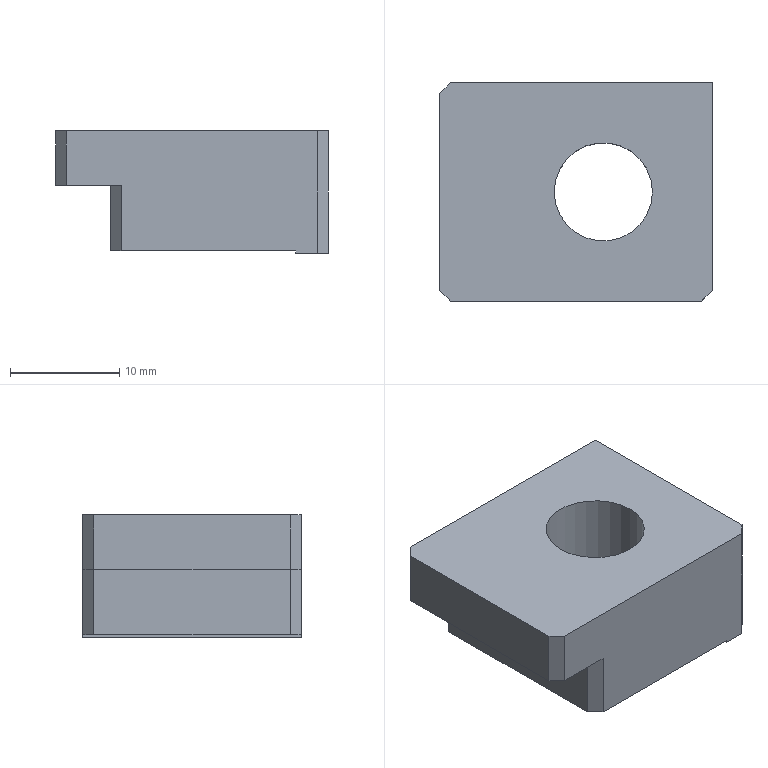Part | NX | features solid 2 | 1 solid | 16 faces | box 25 x 20 x 11.2 mm | volume 4196 mm3 | plane 15 | cylinder 1 | commonest cylinder face diameters 9 x1
STEP:
#1=CARTESIAN_POINT('',(192.5,-300.,61.));
#2=VERTEX_POINT('',#1);
#3=CARTESIAN_POINT('',(197.,-300.,61.));
#4=DIRECTION('',(0.,0.,-1.));
#5=DIRECTION('',(-1.,0.,0.));
#6=AXIS2_PLACEMENT_3D('',#3,#4,#5);
#7=CIRCLE('',#6,4.5);
#8=EDGE_CURVE('',#2,#2,#7,.T.);
#9=ORIENTED_EDGE('',*,*,#8,.F.);
#10=EDGE_LOOP('',(#9));
#11=FACE_BOUND('',#10,.T.);
#12=CARTESIAN_POINT('',(201.5,-300.,50.));
#13=VERTEX_POINT('',#12);
#14=CARTESIAN_POINT('',(197.,-300.,50.));
#15=DIRECTION('',(0.,0.,1.));
#16=DIRECTION('',(1.,0.,0.));
#17=AXIS2_PLACEMENT_3D('',#14,#15,#16);
#18=CIRCLE('',#17,4.5);
#19=EDGE_CURVE('',#13,#13,#18,.T.);
#20=ORIENTED_EDGE('',*,*,#19,.F.);
#21=EDGE_LOOP('',(#20));
#22=FACE_BOUND('',#21,.T.);
#23=CARTESIAN_POINT('',(197.,-300.,10.));
#24=DIRECTION('',(0.,0.,-1.));
#25=DIRECTION('',(-1.,0.,0.));
#26=AXIS2_PLACEMENT_3D('',#23,#24,#25);
#27=CYLINDRICAL_SURFACE('',#26,4.5);
#28=ADVANCED_FACE('',(#11,#22),#27,.F.);
#29=CARTESIAN_POINT('',(182.,-291.,61.));
#30=VERTEX_POINT('',#29);
#31=CARTESIAN_POINT('',(182.,-309.,61.));
#32=VERTEX_POINT('',#31);
#33=CARTESIAN_POINT('',(182.,-268.675,61.));
#34=DIRECTION('',(0.,-1.,0.));
#35=VECTOR('',#34,1000.);
#36=LINE('',#33,#35);
#37=EDGE_CURVE('',#30,#32,#36,.T.);
#38=ORIENTED_EDGE('',*,*,#37,.T.);
#39=CARTESIAN_POINT('',(183.,-310.,61.));
#40=VERTEX_POINT('',#39);
#41=CARTESIAN_POINT('',(182.,-309.,61.));
#42=DIRECTION('',(0.7071,-0.7071,0.));
#43=VECTOR('',#42,1000.);
#44=LINE('',#41,#43);
#45=EDGE_CURVE('',#32,#40,#44,.T.);
#46=ORIENTED_EDGE('',*,*,#45,.T.);
#47=CARTESIAN_POINT('',(206.,-310.,61.));
#48=VERTEX_POINT('',#47);
#49=CARTESIAN_POINT('',(170.325,-310.,61.));
#50=DIRECTION('',(-1.,0.,0.));
#51=VECTOR('',#50,1000.);
#52=LINE('',#49,#51);
#53=EDGE_CURVE('',#48,#40,#52,.T.);
#54=ORIENTED_EDGE('',*,*,#53,.F.);
#55=CARTESIAN_POINT('',(207.,-309.,61.));
#56=VERTEX_POINT('',#55);
#57=CARTESIAN_POINT('',(206.,-310.,61.));
#58=DIRECTION('',(0.7071,0.7071,0.));
#59=VECTOR('',#58,1000.);
#60=LINE('',#57,#59);
#61=EDGE_CURVE('',#48,#56,#60,.T.);
#62=ORIENTED_EDGE('',*,*,#61,.T.);
#63=CARTESIAN_POINT('',(207.,-290.,61.));
#64=VERTEX_POINT('',#63);
#65=CARTESIAN_POINT('',(207.,-268.675,61.));
#66=DIRECTION('',(0.,1.,0.));
#67=VECTOR('',#66,1000.);
#68=LINE('',#65,#67);
#69=EDGE_CURVE('',#56,#64,#68,.T.);
#70=ORIENTED_EDGE('',*,*,#69,.T.);
#71=CARTESIAN_POINT('',(183.,-290.,61.));
#72=VERTEX_POINT('',#71);
#73=CARTESIAN_POINT('',(170.325,-290.,61.));
#74=DIRECTION('',(-1.,0.,0.));
#75=VECTOR('',#74,1000.);
#76=LINE('',#73,#75);
#77=EDGE_CURVE('',#64,#72,#76,.T.);
#78=ORIENTED_EDGE('',*,*,#77,.T.);
#79=CARTESIAN_POINT('',(182.,-291.,61.));
#80=DIRECTION('',(-0.7071,-0.7071,0.));
#81=VECTOR('',#80,1000.);
#82=LINE('',#79,#81);
#83=EDGE_CURVE('',#72,#30,#82,.T.);
#84=ORIENTED_EDGE('',*,*,#83,.T.);
#85=EDGE_LOOP('',(#38,#46,#54,#62,#70,#78,#84));
#86=FACE_BOUND('',#85,.T.);
#87=ORIENTED_EDGE('',*,*,#8,.T.);
#88=EDGE_LOOP('',(#87));
#89=FACE_BOUND('',#88,.T.);
#90=CARTESIAN_POINT('',(170.325,-268.675,61.));
#91=DIRECTION('',(0.,0.,-1.));
#92=DIRECTION('',(-0.7071,-0.7071,0.));
#93=AXIS2_PLACEMENT_3D('',#90,#91,#92);
#94=PLANE('',#93);
#95=ADVANCED_FACE('',(#86,#89),#94,.F.);
#96=ORIENTED_EDGE('',*,*,#83,.F.);
#97=CARTESIAN_POINT('',(183.,-290.,56.));
#98=VERTEX_POINT('',#97);
#99=CARTESIAN_POINT('',(183.,-290.,57.5));
#100=DIRECTION('',(0.,0.,1.));
#101=VECTOR('',#100,1000.);
#102=LINE('',#99,#101);
#103=EDGE_CURVE('',#98,#72,#102,.T.);
#104=ORIENTED_EDGE('',*,*,#103,.F.);
#105=CARTESIAN_POINT('',(182.,-291.,56.));
#106=VERTEX_POINT('',#105);
#107=CARTESIAN_POINT('',(182.,-291.,56.));
#108=DIRECTION('',(0.7071,0.7071,0.));
#109=VECTOR('',#108,1000.);
#110=LINE('',#107,#109);
#111=EDGE_CURVE('',#106,#98,#110,.T.);
#112=ORIENTED_EDGE('',*,*,#111,.F.);
#113=CARTESIAN_POINT('',(182.,-291.,60.));
#114=DIRECTION('',(0.,0.,-1.));
#115=VECTOR('',#114,1000.);
#116=LINE('',#113,#115);
#117=EDGE_CURVE('',#30,#106,#116,.T.);
#118=ORIENTED_EDGE('',*,*,#117,.F.);
#119=EDGE_LOOP('',(#96,#104,#112,#118));
#120=FACE_BOUND('',#119,.T.);
#121=CARTESIAN_POINT('',(182.,-291.,60.));
#122=DIRECTION('',(0.7071,-0.7071,0.));
#123=DIRECTION('',(0.,0.,-1.));
#124=AXIS2_PLACEMENT_3D('',#121,#122,#123);
#125=PLANE('',#124);
#126=ADVANCED_FACE('',(#120),#125,.F.);
#127=CARTESIAN_POINT('',(183.,-310.,56.));
#128=VERTEX_POINT('',#127);
#129=CARTESIAN_POINT('',(182.,-309.,56.));
#130=VERTEX_POINT('',#129);
#131=CARTESIAN_POINT('',(182.,-309.,56.));
#132=DIRECTION('',(-0.7071,0.7071,0.));
#133=VECTOR('',#132,1000.);
#134=LINE('',#131,#133);
#135=EDGE_CURVE('',#128,#130,#134,.T.);
#136=ORIENTED_EDGE('',*,*,#135,.F.);
#137=CARTESIAN_POINT('',(183.,-310.,56.3));
#138=DIRECTION('',(0.,0.,-1.));
#139=VECTOR('',#138,1000.);
#140=LINE('',#137,#139);
#141=EDGE_CURVE('',#40,#128,#140,.T.);
#142=ORIENTED_EDGE('',*,*,#141,.F.);
#143=ORIENTED_EDGE('',*,*,#45,.F.);
#144=CARTESIAN_POINT('',(182.,-309.,64.8));
#145=DIRECTION('',(0.,0.,1.));
#146=VECTOR('',#145,1000.);
#147=LINE('',#144,#146);
#148=EDGE_CURVE('',#130,#32,#147,.T.);
#149=ORIENTED_EDGE('',*,*,#148,.F.);
#150=EDGE_LOOP('',(#136,#142,#143,#149));
#151=FACE_BOUND('',#150,.T.);
#152=CARTESIAN_POINT('',(182.,-309.,60.));
#153=DIRECTION('',(-0.7071,-0.7071,0.));
#154=DIRECTION('',(0.,0.,-1.));
#155=AXIS2_PLACEMENT_3D('',#152,#153,#154);
#156=PLANE('',#155);
#157=ADVANCED_FACE('',(#151),#156,.T.);
#158=CARTESIAN_POINT('',(182.,-306.5,56.));
#159=DIRECTION('',(0.,1.,0.));
#160=VECTOR('',#159,1000.);
#161=LINE('',#158,#160);
#162=EDGE_CURVE('',#130,#106,#161,.T.);
#163=ORIENTED_EDGE('',*,*,#162,.F.);
#164=ORIENTED_EDGE('',*,*,#148,.T.);
#165=ORIENTED_EDGE('',*,*,#37,.F.);
#166=ORIENTED_EDGE('',*,*,#117,.T.);
#167=EDGE_LOOP('',(#163,#164,#165,#166));
#168=FACE_BOUND('',#167,.T.);
#169=CARTESIAN_POINT('',(182.,-310.5,60.));
#170=DIRECTION('',(1.,0.,0.));
#171=DIRECTION('',(0.,0.,-1.));
#172=AXIS2_PLACEMENT_3D('',#169,#170,#171);
#173=PLANE('',#172);
#174=ADVANCED_FACE('',(#168),#173,.F.);
#175=CARTESIAN_POINT('',(188.,-290.,56.));
#176=VERTEX_POINT('',#175);
#177=CARTESIAN_POINT('',(190.,-290.,56.));
#178=DIRECTION('',(1.,0.,0.));
#179=VECTOR('',#178,1000.);
#180=LINE('',#177,#179);
#181=EDGE_CURVE('',#98,#176,#180,.T.);
#182=ORIENTED_EDGE('',*,*,#181,.T.);
#183=CARTESIAN_POINT('',(187.,-291.,56.));
#184=VERTEX_POINT('',#183);
#185=CARTESIAN_POINT('',(179.5,-298.5,56.));
#186=DIRECTION('',(-0.7071,-0.7071,0.));
#187=VECTOR('',#186,1000.);
#188=LINE('',#185,#187);
#189=EDGE_CURVE('',#176,#184,#188,.T.);
#190=ORIENTED_EDGE('',*,*,#189,.T.);
#191=CARTESIAN_POINT('',(187.,-309.,56.));
#192=VERTEX_POINT('',#191);
#193=CARTESIAN_POINT('',(187.,-306.5,56.));
#194=DIRECTION('',(0.,-1.,0.));
#195=VECTOR('',#194,1000.);
#196=LINE('',#193,#195);
#197=EDGE_CURVE('',#184,#192,#196,.T.);
#198=ORIENTED_EDGE('',*,*,#197,.T.);
#199=CARTESIAN_POINT('',(188.,-310.,56.));
#200=VERTEX_POINT('',#199);
#201=CARTESIAN_POINT('',(186.,-308.,56.));
#202=DIRECTION('',(0.7071,-0.7071,0.));
#203=VECTOR('',#202,1000.);
#204=LINE('',#201,#203);
#205=EDGE_CURVE('',#192,#200,#204,.T.);
#206=ORIENTED_EDGE('',*,*,#205,.T.);
#207=CARTESIAN_POINT('',(188.,-310.,56.));
#208=DIRECTION('',(-1.,0.,0.));
#209=VECTOR('',#208,1000.);
#210=LINE('',#207,#209);
#211=EDGE_CURVE('',#200,#128,#210,.T.);
#212=ORIENTED_EDGE('',*,*,#211,.T.);
#213=ORIENTED_EDGE('',*,*,#135,.T.);
#214=ORIENTED_EDGE('',*,*,#162,.T.);
#215=ORIENTED_EDGE('',*,*,#111,.T.);
#216=EDGE_LOOP('',(#182,#190,#198,#206,#212,#213,#214,#215));
#217=FACE_BOUND('',#216,.T.);
#218=CARTESIAN_POINT('',(190.,-306.5,56.));
#219=DIRECTION('',(0.,0.,1.));
#220=DIRECTION('',(1.,0.,0.));
#221=AXIS2_PLACEMENT_3D('',#218,#219,#220);
#222=PLANE('',#221);
#223=ADVANCED_FACE('',(#217),#222,.F.);
#224=CARTESIAN_POINT('',(207.,-290.,49.8));
#225=VERTEX_POINT('',#224);
#226=CARTESIAN_POINT('',(207.,-290.,57.5));
#227=DIRECTION('',(0.,0.,-1.));
#228=VECTOR('',#227,1000.);
#229=LINE('',#226,#228);
#230=EDGE_CURVE('',#64,#225,#229,.T.);
#231=ORIENTED_EDGE('',*,*,#230,.T.);
#232=CARTESIAN_POINT('',(204.,-290.,49.8));
#233=VERTEX_POINT('',#232);
#234=CARTESIAN_POINT('',(195.,-290.,49.8));
#235=DIRECTION('',(1.,0.,0.));
#236=VECTOR('',#235,1000.);
#237=LINE('',#234,#236);
#238=EDGE_CURVE('',#233,#225,#237,.T.);
#239=ORIENTED_EDGE('',*,*,#238,.F.);
#240=CARTESIAN_POINT('',(204.,-290.,50.));
#241=VERTEX_POINT('',#240);
#242=CARTESIAN_POINT('',(204.,-290.,57.5));
#243=DIRECTION('',(0.,0.,1.));
#244=VECTOR('',#243,1000.);
#245=LINE('',#242,#244);
#246=EDGE_CURVE('',#233,#241,#245,.T.);
#247=ORIENTED_EDGE('',*,*,#246,.T.);
#248=CARTESIAN_POINT('',(188.,-290.,50.));
#249=VERTEX_POINT('',#248);
#250=CARTESIAN_POINT('',(190.,-290.,50.));
#251=DIRECTION('',(1.,0.,0.));
#252=VECTOR('',#251,1000.);
#253=LINE('',#250,#252);
#254=EDGE_CURVE('',#249,#241,#253,.T.);
#255=ORIENTED_EDGE('',*,*,#254,.F.);
#256=CARTESIAN_POINT('',(188.,-290.,57.5));
#257=DIRECTION('',(0.,0.,1.));
#258=VECTOR('',#257,1000.);
#259=LINE('',#256,#258);
#260=EDGE_CURVE('',#249,#176,#259,.T.);
#261=ORIENTED_EDGE('',*,*,#260,.T.);
#262=ORIENTED_EDGE('',*,*,#181,.F.);
#263=ORIENTED_EDGE('',*,*,#103,.T.);
#264=ORIENTED_EDGE('',*,*,#77,.F.);
#265=EDGE_LOOP('',(#231,#239,#247,#255,#261,#262,#263,#264));
#266=FACE_BOUND('',#265,.T.);
#267=CARTESIAN_POINT('',(188.,-290.,57.5));
#268=DIRECTION('',(0.,-1.,0.));
#269=DIRECTION('',(0.,0.,-1.));
#270=AXIS2_PLACEMENT_3D('',#267,#268,#269);
#271=PLANE('',#270);
#272=ADVANCED_FACE('',(#266),#271,.F.);
#273=CARTESIAN_POINT('',(206.,-310.,49.8));
#274=VERTEX_POINT('',#273);
#275=CARTESIAN_POINT('',(206.,-310.,64.8));
#276=DIRECTION('',(0.,0.,1.));
#277=VECTOR('',#276,1000.);
#278=LINE('',#275,#277);
#279=EDGE_CURVE('',#274,#48,#278,.T.);
#280=ORIENTED_EDGE('',*,*,#279,.F.);
#281=CARTESIAN_POINT('',(207.,-309.,49.8));
#282=VERTEX_POINT('',#281);
#283=CARTESIAN_POINT('',(206.,-310.,49.8));
#284=DIRECTION('',(-0.7071,-0.7071,0.));
#285=VECTOR('',#284,1000.);
#286=LINE('',#283,#285);
#287=EDGE_CURVE('',#282,#274,#286,.T.);
#288=ORIENTED_EDGE('',*,*,#287,.F.);
#289=CARTESIAN_POINT('',(207.,-309.,49.8));
#290=DIRECTION('',(0.,0.,-1.));
#291=VECTOR('',#290,1000.);
#292=LINE('',#289,#291);
#293=EDGE_CURVE('',#56,#282,#292,.T.);
#294=ORIENTED_EDGE('',*,*,#293,.F.);
#295=ORIENTED_EDGE('',*,*,#61,.F.);
#296=EDGE_LOOP('',(#280,#288,#294,#295));
#297=FACE_BOUND('',#296,.T.);
#298=CARTESIAN_POINT('',(206.,-310.,57.5));
#299=DIRECTION('',(0.7071,-0.7071,0.));
#300=DIRECTION('',(0.,0.,-1.));
#301=AXIS2_PLACEMENT_3D('',#298,#299,#300);
#302=PLANE('',#301);
#303=ADVANCED_FACE('',(#297),#302,.T.);
#304=ORIENTED_EDGE('',*,*,#211,.F.);
#305=CARTESIAN_POINT('',(188.,-310.,50.));
#306=VERTEX_POINT('',#305);
#307=CARTESIAN_POINT('',(188.,-310.,50.));
#308=DIRECTION('',(0.,0.,-1.));
#309=VECTOR('',#308,1000.);
#310=LINE('',#307,#309);
#311=EDGE_CURVE('',#200,#306,#310,.T.);
#312=ORIENTED_EDGE('',*,*,#311,.T.);
#313=CARTESIAN_POINT('',(204.,-310.,50.));
#314=VERTEX_POINT('',#313);
#315=CARTESIAN_POINT('',(190.,-310.,50.));
#316=DIRECTION('',(1.,0.,0.));
#317=VECTOR('',#316,1000.);
#318=LINE('',#315,#317);
#319=EDGE_CURVE('',#306,#314,#318,.T.);
#320=ORIENTED_EDGE('',*,*,#319,.T.);
#321=CARTESIAN_POINT('',(204.,-310.,49.8));
#322=VERTEX_POINT('',#321);
#323=CARTESIAN_POINT('',(204.,-310.,57.5));
#324=DIRECTION('',(0.,0.,1.));
#325=VECTOR('',#324,1000.);
#326=LINE('',#323,#325);
#327=EDGE_CURVE('',#322,#314,#326,.T.);
#328=ORIENTED_EDGE('',*,*,#327,.F.);
#329=CARTESIAN_POINT('',(195.,-310.,49.8));
#330=DIRECTION('',(1.,0.,0.));
#331=VECTOR('',#330,1000.);
#332=LINE('',#329,#331);
#333=EDGE_CURVE('',#322,#274,#332,.T.);
#334=ORIENTED_EDGE('',*,*,#333,.T.);
#335=ORIENTED_EDGE('',*,*,#279,.T.);
#336=ORIENTED_EDGE('',*,*,#53,.T.);
#337=ORIENTED_EDGE('',*,*,#141,.T.);
#338=EDGE_LOOP('',(#304,#312,#320,#328,#334,#335,#336,#337));
#339=FACE_BOUND('',#338,.T.);
#340=CARTESIAN_POINT('',(188.,-310.,57.5));
#341=DIRECTION('',(0.,-1.,0.));
#342=DIRECTION('',(0.,0.,-1.));
#343=AXIS2_PLACEMENT_3D('',#340,#341,#342);
#344=PLANE('',#343);
#345=ADVANCED_FACE('',(#339),#344,.T.);
#346=ORIENTED_EDGE('',*,*,#293,.T.);
#347=CARTESIAN_POINT('',(207.,-306.5,49.8));
#348=DIRECTION('',(0.,1.,0.));
#349=VECTOR('',#348,1000.);
#350=LINE('',#347,#349);
#351=EDGE_CURVE('',#282,#225,#350,.T.);
#352=ORIENTED_EDGE('',*,*,#351,.T.);
#353=ORIENTED_EDGE('',*,*,#230,.F.);
#354=ORIENTED_EDGE('',*,*,#69,.F.);
#355=EDGE_LOOP('',(#346,#352,#353,#354));
#356=FACE_BOUND('',#355,.T.);
#357=CARTESIAN_POINT('',(207.,-306.5,51.5));
#358=DIRECTION('',(-1.,0.,0.));
#359=DIRECTION('',(0.,0.,1.));
#360=AXIS2_PLACEMENT_3D('',#357,#358,#359);
#361=PLANE('',#360);
#362=ADVANCED_FACE('',(#356),#361,.F.);
#363=ORIENTED_EDGE('',*,*,#327,.T.);
#364=CARTESIAN_POINT('',(204.,-306.5,50.));
#365=DIRECTION('',(0.,1.,0.));
#366=VECTOR('',#365,1000.);
#367=LINE('',#364,#366);
#368=EDGE_CURVE('',#314,#241,#367,.T.);
#369=ORIENTED_EDGE('',*,*,#368,.T.);
#370=ORIENTED_EDGE('',*,*,#246,.F.);
#371=CARTESIAN_POINT('',(204.,-306.5,49.8));
#372=DIRECTION('',(0.,1.,0.));
#373=VECTOR('',#372,1000.);
#374=LINE('',#371,#373);
#375=EDGE_CURVE('',#322,#233,#374,.T.);
#376=ORIENTED_EDGE('',*,*,#375,.F.);
#377=EDGE_LOOP('',(#363,#369,#370,#376));
#378=FACE_BOUND('',#377,.T.);
#379=CARTESIAN_POINT('',(204.,-300.,55.75));
#380=DIRECTION('',(1.,0.,0.));
#381=DIRECTION('',(0.,0.,-1.));
#382=AXIS2_PLACEMENT_3D('',#379,#380,#381);
#383=PLANE('',#382);
#384=ADVANCED_FACE('',(#378),#383,.F.);
#385=ORIENTED_EDGE('',*,*,#238,.T.);
#386=ORIENTED_EDGE('',*,*,#351,.F.);
#387=ORIENTED_EDGE('',*,*,#287,.T.);
#388=ORIENTED_EDGE('',*,*,#333,.F.);
#389=ORIENTED_EDGE('',*,*,#375,.T.);
#390=EDGE_LOOP('',(#385,#386,#387,#388,#389));
#391=FACE_BOUND('',#390,.T.);
#392=CARTESIAN_POINT('',(195.,-306.5,49.8));
#393=DIRECTION('',(0.,0.,1.));
#394=DIRECTION('',(1.,0.,0.));
#395=AXIS2_PLACEMENT_3D('',#392,#393,#394);
#396=PLANE('',#395);
#397=ADVANCED_FACE('',(#391),#396,.F.);
#398=ORIENTED_EDGE('',*,*,#319,.F.);
#399=CARTESIAN_POINT('',(187.,-309.,50.));
#400=VERTEX_POINT('',#399);
#401=CARTESIAN_POINT('',(188.,-310.,50.));
#402=DIRECTION('',(-0.7071,0.7071,0.));
#403=VECTOR('',#402,1000.);
#404=LINE('',#401,#403);
#405=EDGE_CURVE('',#306,#400,#404,.T.);
#406=ORIENTED_EDGE('',*,*,#405,.T.);
#407=CARTESIAN_POINT('',(187.,-291.,50.));
#408=VERTEX_POINT('',#407);
#409=CARTESIAN_POINT('',(187.,-306.5,50.));
#410=DIRECTION('',(0.,1.,0.));
#411=VECTOR('',#410,1000.);
#412=LINE('',#409,#411);
#413=EDGE_CURVE('',#400,#408,#412,.T.);
#414=ORIENTED_EDGE('',*,*,#413,.T.);
#415=CARTESIAN_POINT('',(187.,-291.,50.));
#416=DIRECTION('',(0.7071,0.7071,0.));
#417=VECTOR('',#416,1000.);
#418=LINE('',#415,#417);
#419=EDGE_CURVE('',#408,#249,#418,.T.);
#420=ORIENTED_EDGE('',*,*,#419,.T.);
#421=ORIENTED_EDGE('',*,*,#254,.T.);
#422=ORIENTED_EDGE('',*,*,#368,.F.);
#423=EDGE_LOOP('',(#398,#406,#414,#420,#421,#422));
#424=FACE_BOUND('',#423,.T.);
#425=ORIENTED_EDGE('',*,*,#19,.T.);
#426=EDGE_LOOP('',(#425));
#427=FACE_BOUND('',#426,.T.);
#428=CARTESIAN_POINT('',(190.,-306.5,50.));
#429=DIRECTION('',(0.,0.,1.));
#430=DIRECTION('',(1.,0.,0.));
#431=AXIS2_PLACEMENT_3D('',#428,#429,#430);
#432=PLANE('',#431);
#433=ADVANCED_FACE('',(#424,#427),#432,.F.);
#434=ORIENTED_EDGE('',*,*,#189,.F.);
#435=ORIENTED_EDGE('',*,*,#260,.F.);
#436=ORIENTED_EDGE('',*,*,#419,.F.);
#437=CARTESIAN_POINT('',(187.,-291.,57.5));
#438=DIRECTION('',(0.,0.,-1.));
#439=VECTOR('',#438,1000.);
#440=LINE('',#437,#439);
#441=EDGE_CURVE('',#184,#408,#440,.T.);
#442=ORIENTED_EDGE('',*,*,#441,.F.);
#443=EDGE_LOOP('',(#434,#435,#436,#442));
#444=FACE_BOUND('',#443,.T.);
#445=CARTESIAN_POINT('',(187.,-291.,57.5));
#446=DIRECTION('',(0.7071,-0.7071,0.));
#447=DIRECTION('',(0.,0.,-1.));
#448=AXIS2_PLACEMENT_3D('',#445,#446,#447);
#449=PLANE('',#448);
#450=ADVANCED_FACE('',(#444),#449,.F.);
#451=ORIENTED_EDGE('',*,*,#205,.F.);
#452=CARTESIAN_POINT('',(187.,-309.,56.3));
#453=DIRECTION('',(0.,0.,1.));
#454=VECTOR('',#453,1000.);
#455=LINE('',#452,#454);
#456=EDGE_CURVE('',#400,#192,#455,.T.);
#457=ORIENTED_EDGE('',*,*,#456,.F.);
#458=ORIENTED_EDGE('',*,*,#405,.F.);
#459=ORIENTED_EDGE('',*,*,#311,.F.);
#460=EDGE_LOOP('',(#451,#457,#458,#459));
#461=FACE_BOUND('',#460,.T.);
#462=CARTESIAN_POINT('',(188.,-310.,57.5));
#463=DIRECTION('',(-0.7071,-0.7071,0.));
#464=DIRECTION('',(0.,0.,1.));
#465=AXIS2_PLACEMENT_3D('',#462,#463,#464);
#466=PLANE('',#465);
#467=ADVANCED_FACE('',(#461),#466,.T.);
#468=ORIENTED_EDGE('',*,*,#413,.F.);
#469=ORIENTED_EDGE('',*,*,#456,.T.);
#470=ORIENTED_EDGE('',*,*,#197,.F.);
#471=ORIENTED_EDGE('',*,*,#441,.T.);
#472=EDGE_LOOP('',(#468,#469,#470,#471));
#473=FACE_BOUND('',#472,.T.);
#474=CARTESIAN_POINT('',(187.,-306.5,57.5));
#475=DIRECTION('',(1.,0.,0.));
#476=DIRECTION('',(0.,0.,-1.));
#477=AXIS2_PLACEMENT_3D('',#474,#475,#476);
#478=PLANE('',#477);
#479=ADVANCED_FACE('',(#473),#478,.F.);
#480=CLOSED_SHELL('',(#28,#95,#126,#157,#174,#223,#272,#303,#345,#362,#384,#397,#433,#450,#467,#479));
#481=MANIFOLD_SOLID_BREP('',#480);
#482=(LENGTH_UNIT()NAMED_UNIT(*)SI_UNIT(.MILLI.,.METRE.));
#483=UNCERTAINTY_MEASURE_WITH_UNIT(LENGTH_MEASURE(0.00001),#482,'','');
#484=(NAMED_UNIT(*)PLANE_ANGLE_UNIT()SI_UNIT($,.RADIAN.));
#485=(NAMED_UNIT(*)SI_UNIT($,.STERADIAN.)SOLID_ANGLE_UNIT());
#486=(GEOMETRIC_REPRESENTATION_CONTEXT(3)GLOBAL_UNCERTAINTY_ASSIGNED_CONTEXT((#483))GLOBAL_UNIT_ASSIGNED_CONTEXT((#482,#484,#485))REPRESENTATION_CONTEXT('',''));
#487=ADVANCED_BREP_SHAPE_REPRESENTATION('',(#481),#486);